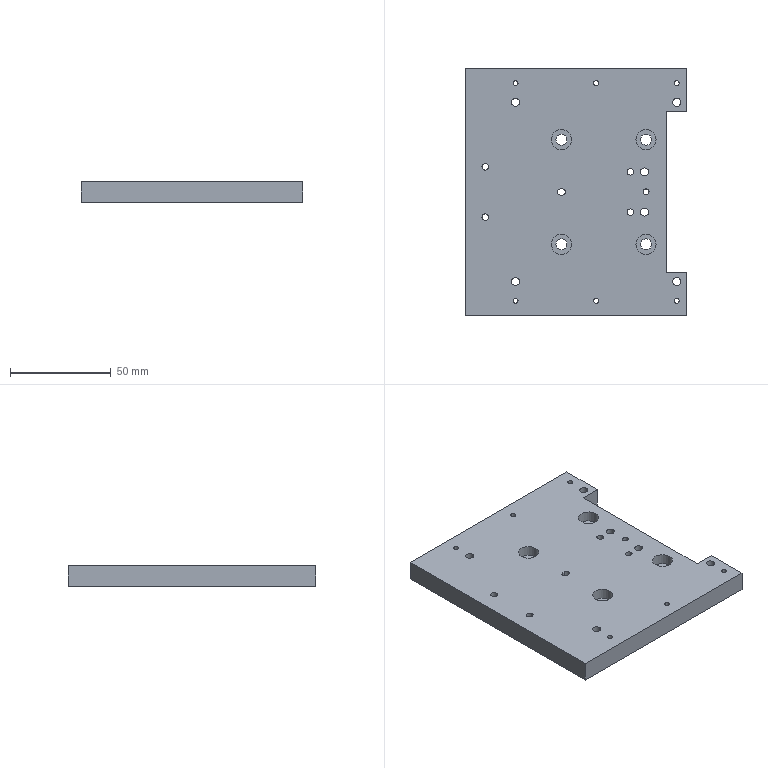Part | 1 solid | 43 faces | box 110 x 123 x 10 mm | volume 123604 mm3 | cylinder 27 | plane 16 | commonest cylinder face diameters 2.5 x6 4 x6 3.3 x4 5.5 x4 10 x4 3 x3
STEP:
#1=CARTESIAN_POINT('',(48.25,60.,10.));
#2=VERTEX_POINT('',#1);
#3=CARTESIAN_POINT('',(48.25,60.,0.));
#4=VERTEX_POINT('',#3);
#5=CARTESIAN_POINT('',(48.25,60.,10.));
#6=DIRECTION('',(0.,0.,-1.));
#7=VECTOR('',#6,1000.);
#8=LINE('',#5,#7);
#9=EDGE_CURVE('',#2,#4,#8,.T.);
#10=ORIENTED_EDGE('',*,*,#9,.T.);
#11=CARTESIAN_POINT('',(47.25,60.,0.));
#12=VERTEX_POINT('',#11);
#13=CARTESIAN_POINT('',(47.25,60.,0.));
#14=DIRECTION('',(1.,0.,0.));
#15=VECTOR('',#14,1000.);
#16=LINE('',#13,#15);
#17=EDGE_CURVE('',#12,#4,#16,.T.);
#18=ORIENTED_EDGE('',*,*,#17,.F.);
#19=CARTESIAN_POINT('',(47.25,60.,10.));
#20=VERTEX_POINT('',#19);
#21=CARTESIAN_POINT('',(47.25,60.,10.));
#22=DIRECTION('',(0.,0.,1.));
#23=VECTOR('',#22,1000.);
#24=LINE('',#21,#23);
#25=EDGE_CURVE('',#12,#20,#24,.T.);
#26=ORIENTED_EDGE('',*,*,#25,.T.);
#27=CARTESIAN_POINT('',(47.25,60.,10.));
#28=DIRECTION('',(1.,0.,0.));
#29=VECTOR('',#28,1000.);
#30=LINE('',#27,#29);
#31=EDGE_CURVE('',#20,#2,#30,.T.);
#32=ORIENTED_EDGE('',*,*,#31,.T.);
#33=EDGE_LOOP('',(#10,#18,#26,#32));
#34=FACE_BOUND('',#33,.T.);
#35=CARTESIAN_POINT('',(47.25,60.,10.));
#36=DIRECTION('',(0.,-1.,0.));
#37=DIRECTION('',(0.,0.,-1.));
#38=AXIS2_PLACEMENT_3D('',#35,#36,#37);
#39=PLANE('',#38);
#40=ADVANCED_FACE('',(#34),#39,.F.);
#41=CARTESIAN_POINT('',(48.25,63.,0.));
#42=VERTEX_POINT('',#41);
#43=CARTESIAN_POINT('',(48.25,63.,10.));
#44=VERTEX_POINT('',#43);
#45=CARTESIAN_POINT('',(48.25,63.,10.));
#46=DIRECTION('',(0.,0.,1.));
#47=VECTOR('',#46,1000.);
#48=LINE('',#45,#47);
#49=EDGE_CURVE('',#42,#44,#48,.T.);
#50=ORIENTED_EDGE('',*,*,#49,.T.);
#51=CARTESIAN_POINT('',(47.25,63.,10.));
#52=VERTEX_POINT('',#51);
#53=CARTESIAN_POINT('',(47.25,63.,10.));
#54=DIRECTION('',(1.,0.,0.));
#55=VECTOR('',#54,1000.);
#56=LINE('',#53,#55);
#57=EDGE_CURVE('',#52,#44,#56,.T.);
#58=ORIENTED_EDGE('',*,*,#57,.F.);
#59=CARTESIAN_POINT('',(47.25,63.,0.));
#60=VERTEX_POINT('',#59);
#61=CARTESIAN_POINT('',(47.25,63.,10.));
#62=DIRECTION('',(0.,0.,-1.));
#63=VECTOR('',#62,1000.);
#64=LINE('',#61,#63);
#65=EDGE_CURVE('',#52,#60,#64,.T.);
#66=ORIENTED_EDGE('',*,*,#65,.T.);
#67=CARTESIAN_POINT('',(47.25,63.,0.));
#68=DIRECTION('',(1.,0.,0.));
#69=VECTOR('',#68,1000.);
#70=LINE('',#67,#69);
#71=EDGE_CURVE('',#60,#42,#70,.T.);
#72=ORIENTED_EDGE('',*,*,#71,.T.);
#73=EDGE_LOOP('',(#50,#58,#66,#72));
#74=FACE_BOUND('',#73,.T.);
#75=CARTESIAN_POINT('',(47.25,63.,10.));
#76=DIRECTION('',(0.,1.,0.));
#77=DIRECTION('',(0.,0.,1.));
#78=AXIS2_PLACEMENT_3D('',#75,#76,#77);
#79=PLANE('',#78);
#80=ADVANCED_FACE('',(#74),#79,.F.);
#81=CARTESIAN_POINT('',(47.25,61.5,10.));
#82=DIRECTION('',(0.,0.,1.));
#83=DIRECTION('',(1.,0.,0.));
#84=AXIS2_PLACEMENT_3D('',#81,#82,#83);
#85=CIRCLE('',#84,1.5);
#86=EDGE_CURVE('',#52,#20,#85,.T.);
#87=ORIENTED_EDGE('',*,*,#86,.T.);
#88=ORIENTED_EDGE('',*,*,#25,.F.);
#89=CARTESIAN_POINT('',(47.25,61.5,0.));
#90=DIRECTION('',(0.,0.,1.));
#91=DIRECTION('',(1.,0.,0.));
#92=AXIS2_PLACEMENT_3D('',#89,#90,#91);
#93=CIRCLE('',#92,1.5);
#94=EDGE_CURVE('',#60,#12,#93,.T.);
#95=ORIENTED_EDGE('',*,*,#94,.F.);
#96=ORIENTED_EDGE('',*,*,#65,.F.);
#97=EDGE_LOOP('',(#87,#88,#95,#96));
#98=FACE_BOUND('',#97,.T.);
#99=CARTESIAN_POINT('',(47.25,61.5,10.));
#100=DIRECTION('',(0.,0.,1.));
#101=DIRECTION('',(1.,0.,0.));
#102=AXIS2_PLACEMENT_3D('',#99,#100,#101);
#103=CYLINDRICAL_SURFACE('',#102,1.5);
#104=ADVANCED_FACE('',(#98),#103,.F.);
#105=CARTESIAN_POINT('',(110.,101.5,10.));
#106=VERTEX_POINT('',#105);
#107=CARTESIAN_POINT('',(100.,101.5,10.));
#108=VERTEX_POINT('',#107);
#109=CARTESIAN_POINT('',(110.,101.5,10.));
#110=DIRECTION('',(-1.,0.,0.));
#111=VECTOR('',#110,1000.);
#112=LINE('',#109,#111);
#113=EDGE_CURVE('',#106,#108,#112,.T.);
#114=ORIENTED_EDGE('',*,*,#113,.T.);
#115=CARTESIAN_POINT('',(100.,101.5,0.));
#116=VERTEX_POINT('',#115);
#117=CARTESIAN_POINT('',(100.,101.5,0.));
#118=DIRECTION('',(0.,0.,1.));
#119=VECTOR('',#118,1000.);
#120=LINE('',#117,#119);
#121=EDGE_CURVE('',#116,#108,#120,.T.);
#122=ORIENTED_EDGE('',*,*,#121,.F.);
#123=CARTESIAN_POINT('',(110.,101.5,0.));
#124=VERTEX_POINT('',#123);
#125=CARTESIAN_POINT('',(110.,101.5,0.));
#126=DIRECTION('',(-1.,0.,0.));
#127=VECTOR('',#126,1000.);
#128=LINE('',#125,#127);
#129=EDGE_CURVE('',#124,#116,#128,.T.);
#130=ORIENTED_EDGE('',*,*,#129,.F.);
#131=CARTESIAN_POINT('',(110.,101.5,0.));
#132=DIRECTION('',(0.,0.,1.));
#133=VECTOR('',#132,1000.);
#134=LINE('',#131,#133);
#135=EDGE_CURVE('',#124,#106,#134,.T.);
#136=ORIENTED_EDGE('',*,*,#135,.T.);
#137=EDGE_LOOP('',(#114,#122,#130,#136));
#138=FACE_BOUND('',#137,.T.);
#139=CARTESIAN_POINT('',(110.,101.5,0.));
#140=DIRECTION('',(0.,1.,0.));
#141=DIRECTION('',(0.,0.,1.));
#142=AXIS2_PLACEMENT_3D('',#139,#140,#141);
#143=PLANE('',#142);
#144=ADVANCED_FACE('',(#138),#143,.F.);
#145=CARTESIAN_POINT('',(100.,21.5,10.));
#146=VERTEX_POINT('',#145);
#147=CARTESIAN_POINT('',(100.,101.5,10.));
#148=DIRECTION('',(0.,-1.,0.));
#149=VECTOR('',#148,1000.);
#150=LINE('',#147,#149);
#151=EDGE_CURVE('',#108,#146,#150,.T.);
#152=ORIENTED_EDGE('',*,*,#151,.T.);
#153=CARTESIAN_POINT('',(100.,21.5,0.));
#154=VERTEX_POINT('',#153);
#155=CARTESIAN_POINT('',(100.,21.5,0.));
#156=DIRECTION('',(0.,0.,1.));
#157=VECTOR('',#156,1000.);
#158=LINE('',#155,#157);
#159=EDGE_CURVE('',#154,#146,#158,.T.);
#160=ORIENTED_EDGE('',*,*,#159,.F.);
#161=CARTESIAN_POINT('',(100.,101.5,0.));
#162=DIRECTION('',(0.,-1.,0.));
#163=VECTOR('',#162,1000.);
#164=LINE('',#161,#163);
#165=EDGE_CURVE('',#116,#154,#164,.T.);
#166=ORIENTED_EDGE('',*,*,#165,.F.);
#167=ORIENTED_EDGE('',*,*,#121,.T.);
#168=EDGE_LOOP('',(#152,#160,#166,#167));
#169=FACE_BOUND('',#168,.T.);
#170=CARTESIAN_POINT('',(100.,101.5,0.));
#171=DIRECTION('',(-1.,0.,0.));
#172=DIRECTION('',(0.,0.,1.));
#173=AXIS2_PLACEMENT_3D('',#170,#171,#172);
#174=PLANE('',#173);
#175=ADVANCED_FACE('',(#169),#174,.F.);
#176=CARTESIAN_POINT('',(110.,21.5,10.));
#177=VERTEX_POINT('',#176);
#178=CARTESIAN_POINT('',(110.,21.5,10.));
#179=DIRECTION('',(1.,0.,0.));
#180=VECTOR('',#179,1000.);
#181=LINE('',#178,#180);
#182=EDGE_CURVE('',#146,#177,#181,.T.);
#183=ORIENTED_EDGE('',*,*,#182,.T.);
#184=CARTESIAN_POINT('',(110.,21.5,0.));
#185=VERTEX_POINT('',#184);
#186=CARTESIAN_POINT('',(110.,21.5,0.));
#187=DIRECTION('',(0.,0.,1.));
#188=VECTOR('',#187,1000.);
#189=LINE('',#186,#188);
#190=EDGE_CURVE('',#185,#177,#189,.T.);
#191=ORIENTED_EDGE('',*,*,#190,.F.);
#192=CARTESIAN_POINT('',(110.,21.5,0.));
#193=DIRECTION('',(1.,0.,0.));
#194=VECTOR('',#193,1000.);
#195=LINE('',#192,#194);
#196=EDGE_CURVE('',#154,#185,#195,.T.);
#197=ORIENTED_EDGE('',*,*,#196,.F.);
#198=ORIENTED_EDGE('',*,*,#159,.T.);
#199=EDGE_LOOP('',(#183,#191,#197,#198));
#200=FACE_BOUND('',#199,.T.);
#201=CARTESIAN_POINT('',(110.,21.5,0.));
#202=DIRECTION('',(0.,-1.,0.));
#203=DIRECTION('',(0.,0.,-1.));
#204=AXIS2_PLACEMENT_3D('',#201,#202,#203);
#205=PLANE('',#204);
#206=ADVANCED_FACE('',(#200),#205,.F.);
#207=CARTESIAN_POINT('',(52.75,87.5,4.6));
#208=VERTEX_POINT('',#207);
#209=CARTESIAN_POINT('',(47.75,87.5,4.6));
#210=DIRECTION('',(0.,0.,1.));
#211=DIRECTION('',(1.,0.,0.));
#212=AXIS2_PLACEMENT_3D('',#209,#210,#211);
#213=CIRCLE('',#212,5.);
#214=EDGE_CURVE('',#208,#208,#213,.T.);
#215=ORIENTED_EDGE('',*,*,#214,.T.);
#216=EDGE_LOOP('',(#215));
#217=FACE_BOUND('',#216,.T.);
#218=CARTESIAN_POINT('',(50.5,87.5,4.6));
#219=VERTEX_POINT('',#218);
#220=CARTESIAN_POINT('',(47.75,87.5,4.6));
#221=DIRECTION('',(0.,0.,1.));
#222=DIRECTION('',(1.,0.,0.));
#223=AXIS2_PLACEMENT_3D('',#220,#221,#222);
#224=CIRCLE('',#223,2.75);
#225=EDGE_CURVE('',#219,#219,#224,.T.);
#226=ORIENTED_EDGE('',*,*,#225,.F.);
#227=EDGE_LOOP('',(#226));
#228=FACE_BOUND('',#227,.T.);
#229=CARTESIAN_POINT('',(50.5,87.5,4.6));
#230=DIRECTION('',(0.,0.,-1.));
#231=DIRECTION('',(-1.,0.,0.));
#232=AXIS2_PLACEMENT_3D('',#229,#230,#231);
#233=PLANE('',#232);
#234=ADVANCED_FACE('',(#217,#228),#233,.F.);
#235=CARTESIAN_POINT('',(42.75,35.5,4.6));
#236=VERTEX_POINT('',#235);
#237=CARTESIAN_POINT('',(47.75,35.5,4.6));
#238=DIRECTION('',(0.,0.,1.));
#239=DIRECTION('',(-1.,0.,0.));
#240=AXIS2_PLACEMENT_3D('',#237,#238,#239);
#241=CIRCLE('',#240,5.);
#242=EDGE_CURVE('',#236,#236,#241,.T.);
#243=ORIENTED_EDGE('',*,*,#242,.T.);
#244=EDGE_LOOP('',(#243));
#245=FACE_BOUND('',#244,.T.);
#246=CARTESIAN_POINT('',(45.,35.5,4.6));
#247=VERTEX_POINT('',#246);
#248=CARTESIAN_POINT('',(47.75,35.5,4.6));
#249=DIRECTION('',(0.,0.,1.));
#250=DIRECTION('',(-1.,0.,0.));
#251=AXIS2_PLACEMENT_3D('',#248,#249,#250);
#252=CIRCLE('',#251,2.75);
#253=EDGE_CURVE('',#247,#247,#252,.T.);
#254=ORIENTED_EDGE('',*,*,#253,.F.);
#255=EDGE_LOOP('',(#254));
#256=FACE_BOUND('',#255,.T.);
#257=CARTESIAN_POINT('',(50.5,87.5,4.6));
#258=DIRECTION('',(0.,0.,-1.));
#259=DIRECTION('',(-1.,0.,0.));
#260=AXIS2_PLACEMENT_3D('',#257,#258,#259);
#261=PLANE('',#260);
#262=ADVANCED_FACE('',(#245,#256),#261,.F.);
#263=CARTESIAN_POINT('',(84.75,87.5,4.6));
#264=VERTEX_POINT('',#263);
#265=CARTESIAN_POINT('',(89.75,87.5,4.6));
#266=DIRECTION('',(0.,0.,1.));
#267=DIRECTION('',(-1.,0.,0.));
#268=AXIS2_PLACEMENT_3D('',#265,#266,#267);
#269=CIRCLE('',#268,5.);
#270=EDGE_CURVE('',#264,#264,#269,.T.);
#271=ORIENTED_EDGE('',*,*,#270,.T.);
#272=EDGE_LOOP('',(#271));
#273=FACE_BOUND('',#272,.T.);
#274=CARTESIAN_POINT('',(87.,87.5,4.6));
#275=VERTEX_POINT('',#274);
#276=CARTESIAN_POINT('',(89.75,87.5,4.6));
#277=DIRECTION('',(0.,0.,1.));
#278=DIRECTION('',(-1.,0.,0.));
#279=AXIS2_PLACEMENT_3D('',#276,#277,#278);
#280=CIRCLE('',#279,2.75);
#281=EDGE_CURVE('',#275,#275,#280,.T.);
#282=ORIENTED_EDGE('',*,*,#281,.F.);
#283=EDGE_LOOP('',(#282));
#284=FACE_BOUND('',#283,.T.);
#285=CARTESIAN_POINT('',(50.5,87.5,4.6));
#286=DIRECTION('',(0.,0.,-1.));
#287=DIRECTION('',(-1.,0.,0.));
#288=AXIS2_PLACEMENT_3D('',#285,#286,#287);
#289=PLANE('',#288);
#290=ADVANCED_FACE('',(#273,#284),#289,.F.);
#291=CARTESIAN_POINT('',(84.75,35.5,4.6));
#292=VERTEX_POINT('',#291);
#293=CARTESIAN_POINT('',(89.75,35.5,4.6));
#294=DIRECTION('',(0.,0.,1.));
#295=DIRECTION('',(-1.,0.,0.));
#296=AXIS2_PLACEMENT_3D('',#293,#294,#295);
#297=CIRCLE('',#296,5.);
#298=EDGE_CURVE('',#292,#292,#297,.T.);
#299=ORIENTED_EDGE('',*,*,#298,.T.);
#300=EDGE_LOOP('',(#299));
#301=FACE_BOUND('',#300,.T.);
#302=CARTESIAN_POINT('',(87.,35.5,4.6));
#303=VERTEX_POINT('',#302);
#304=CARTESIAN_POINT('',(89.75,35.5,4.6));
#305=DIRECTION('',(0.,0.,1.));
#306=DIRECTION('',(-1.,0.,0.));
#307=AXIS2_PLACEMENT_3D('',#304,#305,#306);
#308=CIRCLE('',#307,2.75);
#309=EDGE_CURVE('',#303,#303,#308,.T.);
#310=ORIENTED_EDGE('',*,*,#309,.F.);
#311=EDGE_LOOP('',(#310));
#312=FACE_BOUND('',#311,.T.);
#313=CARTESIAN_POINT('',(50.5,87.5,4.6));
#314=DIRECTION('',(0.,0.,-1.));
#315=DIRECTION('',(-1.,0.,0.));
#316=AXIS2_PLACEMENT_3D('',#313,#314,#315);
#317=PLANE('',#316);
#318=ADVANCED_FACE('',(#301,#312),#317,.F.);
#319=CARTESIAN_POINT('',(110.,123.,0.));
#320=VERTEX_POINT('',#319);
#321=CARTESIAN_POINT('',(0.,123.,0.));
#322=VERTEX_POINT('',#321);
#323=CARTESIAN_POINT('',(0.,123.,0.));
#324=DIRECTION('',(-1.,0.,0.));
#325=VECTOR('',#324,1000.);
#326=LINE('',#323,#325);
#327=EDGE_CURVE('',#320,#322,#326,.T.);
#328=ORIENTED_EDGE('',*,*,#327,.T.);
#329=CARTESIAN_POINT('',(0.,123.,10.));
#330=VERTEX_POINT('',#329);
#331=CARTESIAN_POINT('',(0.,123.,10.));
#332=DIRECTION('',(0.,0.,-1.));
#333=VECTOR('',#332,1000.);
#334=LINE('',#331,#333);
#335=EDGE_CURVE('',#330,#322,#334,.T.);
#336=ORIENTED_EDGE('',*,*,#335,.F.);
#337=CARTESIAN_POINT('',(110.,123.,10.));
#338=VERTEX_POINT('',#337);
#339=CARTESIAN_POINT('',(0.,123.,10.));
#340=DIRECTION('',(-1.,0.,0.));
#341=VECTOR('',#340,1000.);
#342=LINE('',#339,#341);
#343=EDGE_CURVE('',#338,#330,#342,.T.);
#344=ORIENTED_EDGE('',*,*,#343,.F.);
#345=CARTESIAN_POINT('',(110.,123.,10.));
#346=DIRECTION('',(0.,0.,-1.));
#347=VECTOR('',#346,1000.);
#348=LINE('',#345,#347);
#349=EDGE_CURVE('',#338,#320,#348,.T.);
#350=ORIENTED_EDGE('',*,*,#349,.T.);
#351=EDGE_LOOP('',(#328,#336,#344,#350));
#352=FACE_BOUND('',#351,.T.);
#353=CARTESIAN_POINT('',(0.,123.,10.));
#354=DIRECTION('',(0.,-1.,0.));
#355=DIRECTION('',(0.,0.,-1.));
#356=AXIS2_PLACEMENT_3D('',#353,#354,#355);
#357=PLANE('',#356);
#358=ADVANCED_FACE('',(#352),#357,.F.);
#359=CARTESIAN_POINT('',(110.,0.,10.));
#360=DIRECTION('',(0.,1.,0.));
#361=VECTOR('',#360,1000.);
#362=LINE('',#359,#361);
#363=EDGE_CURVE('',#106,#338,#362,.T.);
#364=ORIENTED_EDGE('',*,*,#363,.F.);
#365=ORIENTED_EDGE('',*,*,#135,.F.);
#366=CARTESIAN_POINT('',(110.,0.,0.));
#367=DIRECTION('',(0.,1.,0.));
#368=VECTOR('',#367,1000.);
#369=LINE('',#366,#368);
#370=EDGE_CURVE('',#124,#320,#369,.T.);
#371=ORIENTED_EDGE('',*,*,#370,.T.);
#372=ORIENTED_EDGE('',*,*,#349,.F.);
#373=EDGE_LOOP('',(#364,#365,#371,#372));
#374=FACE_BOUND('',#373,.T.);
#375=CARTESIAN_POINT('',(110.,0.,10.));
#376=DIRECTION('',(-1.,0.,0.));
#377=DIRECTION('',(0.,0.,1.));
#378=AXIS2_PLACEMENT_3D('',#375,#376,#377);
#379=PLANE('',#378);
#380=ADVANCED_FACE('',(#374),#379,.F.);
#381=CARTESIAN_POINT('',(0.,0.,0.));
#382=VERTEX_POINT('',#381);
#383=CARTESIAN_POINT('',(110.,0.,0.));
#384=VERTEX_POINT('',#383);
#385=CARTESIAN_POINT('',(0.,0.,0.));
#386=DIRECTION('',(1.,0.,0.));
#387=VECTOR('',#386,1000.);
#388=LINE('',#385,#387);
#389=EDGE_CURVE('',#382,#384,#388,.T.);
#390=ORIENTED_EDGE('',*,*,#389,.T.);
#391=CARTESIAN_POINT('',(110.,0.,10.));
#392=VERTEX_POINT('',#391);
#393=CARTESIAN_POINT('',(110.,0.,10.));
#394=DIRECTION('',(0.,0.,-1.));
#395=VECTOR('',#394,1000.);
#396=LINE('',#393,#395);
#397=EDGE_CURVE('',#392,#384,#396,.T.);
#398=ORIENTED_EDGE('',*,*,#397,.F.);
#399=CARTESIAN_POINT('',(0.,0.,10.));
#400=VERTEX_POINT('',#399);
#401=CARTESIAN_POINT('',(0.,0.,10.));
#402=DIRECTION('',(1.,0.,0.));
#403=VECTOR('',#402,1000.);
#404=LINE('',#401,#403);
#405=EDGE_CURVE('',#400,#392,#404,.T.);
#406=ORIENTED_EDGE('',*,*,#405,.F.);
#407=CARTESIAN_POINT('',(0.,0.,10.));
#408=DIRECTION('',(0.,0.,-1.));
#409=VECTOR('',#408,1000.);
#410=LINE('',#407,#409);
#411=EDGE_CURVE('',#400,#382,#410,.T.);
#412=ORIENTED_EDGE('',*,*,#411,.T.);
#413=EDGE_LOOP('',(#390,#398,#406,#412));
#414=FACE_BOUND('',#413,.T.);
#415=CARTESIAN_POINT('',(0.,0.,10.));
#416=DIRECTION('',(0.,1.,0.));
#417=DIRECTION('',(0.,0.,1.));
#418=AXIS2_PLACEMENT_3D('',#415,#416,#417);
#419=PLANE('',#418);
#420=ADVANCED_FACE('',(#414),#419,.F.);
#421=CARTESIAN_POINT('',(0.,0.,0.));
#422=DIRECTION('',(0.,-1.,0.));
#423=VECTOR('',#422,1000.);
#424=LINE('',#421,#423);
#425=EDGE_CURVE('',#322,#382,#424,.T.);
#426=ORIENTED_EDGE('',*,*,#425,.T.);
#427=ORIENTED_EDGE('',*,*,#411,.F.);
#428=CARTESIAN_POINT('',(0.,0.,10.));
#429=DIRECTION('',(0.,-1.,0.));
#430=VECTOR('',#429,1000.);
#431=LINE('',#428,#430);
#432=EDGE_CURVE('',#330,#400,#431,.T.);
#433=ORIENTED_EDGE('',*,*,#432,.F.);
#434=ORIENTED_EDGE('',*,*,#335,.T.);
#435=EDGE_LOOP('',(#426,#427,#433,#434));
#436=FACE_BOUND('',#435,.T.);
#437=CARTESIAN_POINT('',(0.,0.,10.));
#438=DIRECTION('',(1.,0.,0.));
#439=DIRECTION('',(0.,0.,-1.));
#440=AXIS2_PLACEMENT_3D('',#437,#438,#439);
#441=PLANE('',#440);
#442=ADVANCED_FACE('',(#436),#441,.F.);
#443=CARTESIAN_POINT('',(94.75,87.5,10.));
#444=VERTEX_POINT('',#443);
#445=CARTESIAN_POINT('',(89.75,87.5,10.));
#446=DIRECTION('',(0.,0.,1.));
#447=DIRECTION('',(1.,0.,0.));
#448=AXIS2_PLACEMENT_3D('',#445,#446,#447);
#449=CIRCLE('',#448,5.);
#450=EDGE_CURVE('',#444,#444,#449,.T.);
#451=ORIENTED_EDGE('',*,*,#450,.F.);
#452=EDGE_LOOP('',(#451));
#453=FACE_BOUND('',#452,.T.);
#454=CARTESIAN_POINT('',(110.,0.,10.));
#455=DIRECTION('',(0.,1.,0.));
#456=VECTOR('',#455,1000.);
#457=LINE('',#454,#456);
#458=EDGE_CURVE('',#392,#177,#457,.T.);
#459=ORIENTED_EDGE('',*,*,#458,.T.);
#460=ORIENTED_EDGE('',*,*,#182,.F.);
#461=ORIENTED_EDGE('',*,*,#151,.F.);
#462=ORIENTED_EDGE('',*,*,#113,.F.);
#463=ORIENTED_EDGE('',*,*,#363,.T.);
#464=ORIENTED_EDGE('',*,*,#343,.T.);
#465=ORIENTED_EDGE('',*,*,#432,.T.);
#466=ORIENTED_EDGE('',*,*,#405,.T.);
#467=EDGE_LOOP('',(#459,#460,#461,#462,#463,#464,#465,#466));
#468=FACE_BOUND('',#467,.T.);
#469=CARTESIAN_POINT('',(106.25,7.5,10.));
#470=VERTEX_POINT('',#469);
#471=CARTESIAN_POINT('',(105.,7.5,10.));
#472=DIRECTION('',(0.,0.,1.));
#473=DIRECTION('',(1.,0.,0.));
#474=AXIS2_PLACEMENT_3D('',#471,#472,#473);
#475=CIRCLE('',#474,1.25);
#476=EDGE_CURVE('',#470,#470,#475,.T.);
#477=ORIENTED_EDGE('',*,*,#476,.F.);
#478=EDGE_LOOP('',(#477));
#479=FACE_BOUND('',#478,.T.);
#480=CARTESIAN_POINT('',(66.25,7.5,10.));
#481=VERTEX_POINT('',#480);
#482=CARTESIAN_POINT('',(65.,7.5,10.));
#483=DIRECTION('',(0.,0.,1.));
#484=DIRECTION('',(1.,0.,0.));
#485=AXIS2_PLACEMENT_3D('',#482,#483,#484);
#486=CIRCLE('',#485,1.25);
#487=EDGE_CURVE('',#481,#481,#486,.T.);
#488=ORIENTED_EDGE('',*,*,#487,.F.);
#489=EDGE_LOOP('',(#488));
#490=FACE_BOUND('',#489,.T.);
#491=CARTESIAN_POINT('',(26.25,7.5,10.));
#492=VERTEX_POINT('',#491);
#493=CARTESIAN_POINT('',(25.,7.5,10.));
#494=DIRECTION('',(0.,0.,1.));
#495=DIRECTION('',(1.,0.,0.));
#496=AXIS2_PLACEMENT_3D('',#493,#494,#495);
#497=CIRCLE('',#496,1.25);
#498=EDGE_CURVE('',#492,#492,#497,.T.);
#499=ORIENTED_EDGE('',*,*,#498,.F.);
#500=EDGE_LOOP('',(#499));
#501=FACE_BOUND('',#500,.T.);
#502=CARTESIAN_POINT('',(26.25,115.5,10.));
#503=VERTEX_POINT('',#502);
#504=CARTESIAN_POINT('',(25.,115.5,10.));
#505=DIRECTION('',(0.,0.,1.));
#506=DIRECTION('',(1.,0.,0.));
#507=AXIS2_PLACEMENT_3D('',#504,#505,#506);
#508=CIRCLE('',#507,1.25);
#509=EDGE_CURVE('',#503,#503,#508,.T.);
#510=ORIENTED_EDGE('',*,*,#509,.F.);
#511=EDGE_LOOP('',(#510));
#512=FACE_BOUND('',#511,.T.);
#513=CARTESIAN_POINT('',(66.25,115.5,10.));
#514=VERTEX_POINT('',#513);
#515=CARTESIAN_POINT('',(65.,115.5,10.));
#516=DIRECTION('',(0.,0.,1.));
#517=DIRECTION('',(1.,0.,0.));
#518=AXIS2_PLACEMENT_3D('',#515,#516,#517);
#519=CIRCLE('',#518,1.25);
#520=EDGE_CURVE('',#514,#514,#519,.T.);
#521=ORIENTED_EDGE('',*,*,#520,.F.);
#522=EDGE_LOOP('',(#521));
#523=FACE_BOUND('',#522,.T.);
#524=CARTESIAN_POINT('',(106.25,115.5,10.));
#525=VERTEX_POINT('',#524);
#526=CARTESIAN_POINT('',(105.,115.5,10.));
#527=DIRECTION('',(0.,0.,1.));
#528=DIRECTION('',(1.,0.,0.));
#529=AXIS2_PLACEMENT_3D('',#526,#527,#528);
#530=CIRCLE('',#529,1.25);
#531=EDGE_CURVE('',#525,#525,#530,.T.);
#532=ORIENTED_EDGE('',*,*,#531,.F.);
#533=EDGE_LOOP('',(#532));
#534=FACE_BOUND('',#533,.T.);
#535=CARTESIAN_POINT('',(94.75,35.5,10.));
#536=VERTEX_POINT('',#535);
#537=CARTESIAN_POINT('',(89.75,35.5,10.));
#538=DIRECTION('',(0.,0.,1.));
#539=DIRECTION('',(1.,0.,0.));
#540=AXIS2_PLACEMENT_3D('',#537,#538,#539);
#541=CIRCLE('',#540,5.);
#542=EDGE_CURVE('',#536,#536,#541,.T.);
#543=ORIENTED_EDGE('',*,*,#542,.F.);
#544=EDGE_LOOP('',(#543));
#545=FACE_BOUND('',#544,.T.);
#546=CARTESIAN_POINT('',(52.75,35.5,10.));
#547=VERTEX_POINT('',#546);
#548=CARTESIAN_POINT('',(47.75,35.5,10.));
#549=DIRECTION('',(0.,0.,1.));
#550=DIRECTION('',(1.,0.,0.));
#551=AXIS2_PLACEMENT_3D('',#548,#549,#550);
#552=CIRCLE('',#551,5.);
#553=EDGE_CURVE('',#547,#547,#552,.T.);
#554=ORIENTED_EDGE('',*,*,#553,.F.);
#555=EDGE_LOOP('',(#554));
#556=FACE_BOUND('',#555,.T.);
#557=CARTESIAN_POINT('',(52.75,87.5,10.));
#558=VERTEX_POINT('',#557);
#559=CARTESIAN_POINT('',(47.75,87.5,10.));
#560=DIRECTION('',(0.,0.,1.));
#561=DIRECTION('',(1.,0.,0.));
#562=AXIS2_PLACEMENT_3D('',#559,#560,#561);
#563=CIRCLE('',#562,5.);
#564=EDGE_CURVE('',#558,#558,#563,.T.);
#565=ORIENTED_EDGE('',*,*,#564,.F.);
#566=EDGE_LOOP('',(#565));
#567=FACE_BOUND('',#566,.T.);
#568=CARTESIAN_POINT('',(11.65,49.,10.));
#569=VERTEX_POINT('',#568);
#570=CARTESIAN_POINT('',(10.,49.,10.));
#571=DIRECTION('',(0.,0.,1.));
#572=DIRECTION('',(1.,0.,0.));
#573=AXIS2_PLACEMENT_3D('',#570,#571,#572);
#574=CIRCLE('',#573,1.65);
#575=EDGE_CURVE('',#569,#569,#574,.T.);
#576=ORIENTED_EDGE('',*,*,#575,.F.);
#577=EDGE_LOOP('',(#576));
#578=FACE_BOUND('',#577,.T.);
#579=CARTESIAN_POINT('',(11.65,74.,10.));
#580=VERTEX_POINT('',#579);
#581=CARTESIAN_POINT('',(10.,74.,10.));
#582=DIRECTION('',(0.,0.,1.));
#583=DIRECTION('',(1.,0.,0.));
#584=AXIS2_PLACEMENT_3D('',#581,#582,#583);
#585=CIRCLE('',#584,1.65);
#586=EDGE_CURVE('',#580,#580,#585,.T.);
#587=ORIENTED_EDGE('',*,*,#586,.F.);
#588=EDGE_LOOP('',(#587));
#589=FACE_BOUND('',#588,.T.);
#590=CARTESIAN_POINT('',(83.65,51.5,10.));
#591=VERTEX_POINT('',#590);
#592=CARTESIAN_POINT('',(82.,51.5,10.));
#593=DIRECTION('',(0.,0.,1.));
#594=DIRECTION('',(1.,0.,0.));
#595=AXIS2_PLACEMENT_3D('',#592,#593,#594);
#596=CIRCLE('',#595,1.65);
#597=EDGE_CURVE('',#591,#591,#596,.T.);
#598=ORIENTED_EDGE('',*,*,#597,.F.);
#599=EDGE_LOOP('',(#598));
#600=FACE_BOUND('',#599,.T.);
#601=CARTESIAN_POINT('',(83.65,71.5,10.));
#602=VERTEX_POINT('',#601);
#603=CARTESIAN_POINT('',(82.,71.5,10.));
#604=DIRECTION('',(0.,0.,1.));
#605=DIRECTION('',(1.,0.,0.));
#606=AXIS2_PLACEMENT_3D('',#603,#604,#605);
#607=CIRCLE('',#606,1.65);
#608=EDGE_CURVE('',#602,#602,#607,.T.);
#609=ORIENTED_EDGE('',*,*,#608,.F.);
#610=EDGE_LOOP('',(#609));
#611=FACE_BOUND('',#610,.T.);
#612=CARTESIAN_POINT('',(91.,51.5,10.));
#613=VERTEX_POINT('',#612);
#614=CARTESIAN_POINT('',(89.,51.5,10.));
#615=DIRECTION('',(0.,0.,1.));
#616=DIRECTION('',(1.,0.,0.));
#617=AXIS2_PLACEMENT_3D('',#614,#615,#616);
#618=CIRCLE('',#617,2.);
#619=EDGE_CURVE('',#613,#613,#618,.T.);
#620=ORIENTED_EDGE('',*,*,#619,.F.);
#621=EDGE_LOOP('',(#620));
#622=FACE_BOUND('',#621,.T.);
#623=CARTESIAN_POINT('',(91.,71.5,10.));
#624=VERTEX_POINT('',#623);
#625=CARTESIAN_POINT('',(89.,71.5,10.));
#626=DIRECTION('',(0.,0.,1.));
#627=DIRECTION('',(1.,0.,0.));
#628=AXIS2_PLACEMENT_3D('',#625,#626,#627);
#629=CIRCLE('',#628,2.);
#630=EDGE_CURVE('',#624,#624,#629,.T.);
#631=ORIENTED_EDGE('',*,*,#630,.F.);
#632=EDGE_LOOP('',(#631));
#633=FACE_BOUND('',#632,.T.);
#634=CARTESIAN_POINT('',(27.,17.,10.));
#635=VERTEX_POINT('',#634);
#636=CARTESIAN_POINT('',(25.,17.,10.));
#637=DIRECTION('',(0.,0.,1.));
#638=DIRECTION('',(1.,0.,0.));
#639=AXIS2_PLACEMENT_3D('',#636,#637,#638);
#640=CIRCLE('',#639,2.);
#641=EDGE_CURVE('',#635,#635,#640,.T.);
#642=ORIENTED_EDGE('',*,*,#641,.F.);
#643=EDGE_LOOP('',(#642));
#644=FACE_BOUND('',#643,.T.);
#645=CARTESIAN_POINT('',(107.,17.,10.));
#646=VERTEX_POINT('',#645);
#647=CARTESIAN_POINT('',(105.,17.,10.));
#648=DIRECTION('',(0.,0.,1.));
#649=DIRECTION('',(1.,0.,0.));
#650=AXIS2_PLACEMENT_3D('',#647,#648,#649);
#651=CIRCLE('',#650,2.);
#652=EDGE_CURVE('',#646,#646,#651,.T.);
#653=ORIENTED_EDGE('',*,*,#652,.F.);
#654=EDGE_LOOP('',(#653));
#655=FACE_BOUND('',#654,.T.);
#656=CARTESIAN_POINT('',(27.,106.,10.));
#657=VERTEX_POINT('',#656);
#658=CARTESIAN_POINT('',(25.,106.,10.));
#659=DIRECTION('',(0.,0.,1.));
#660=DIRECTION('',(1.,0.,0.));
#661=AXIS2_PLACEMENT_3D('',#658,#659,#660);
#662=CIRCLE('',#661,2.);
#663=EDGE_CURVE('',#657,#657,#662,.T.);
#664=ORIENTED_EDGE('',*,*,#663,.F.);
#665=EDGE_LOOP('',(#664));
#666=FACE_BOUND('',#665,.T.);
#667=CARTESIAN_POINT('',(107.,106.,10.));
#668=VERTEX_POINT('',#667);
#669=CARTESIAN_POINT('',(105.,106.,10.));
#670=DIRECTION('',(0.,0.,1.));
#671=DIRECTION('',(1.,0.,0.));
#672=AXIS2_PLACEMENT_3D('',#669,#670,#671);
#673=CIRCLE('',#672,2.);
#674=EDGE_CURVE('',#668,#668,#673,.T.);
#675=ORIENTED_EDGE('',*,*,#674,.F.);
#676=EDGE_LOOP('',(#675));
#677=FACE_BOUND('',#676,.T.);
#678=ORIENTED_EDGE('',*,*,#57,.T.);
#679=CARTESIAN_POINT('',(48.25,61.5,10.));
#680=DIRECTION('',(0.,0.,1.));
#681=DIRECTION('',(1.,0.,0.));
#682=AXIS2_PLACEMENT_3D('',#679,#680,#681);
#683=CIRCLE('',#682,1.5);
#684=EDGE_CURVE('',#2,#44,#683,.T.);
#685=ORIENTED_EDGE('',*,*,#684,.F.);
#686=ORIENTED_EDGE('',*,*,#31,.F.);
#687=ORIENTED_EDGE('',*,*,#86,.F.);
#688=EDGE_LOOP('',(#678,#685,#686,#687));
#689=FACE_BOUND('',#688,.T.);
#690=CARTESIAN_POINT('',(91.25,61.5,10.));
#691=VERTEX_POINT('',#690);
#692=CARTESIAN_POINT('',(89.75,61.5,10.));
#693=DIRECTION('',(0.,0.,1.));
#694=DIRECTION('',(1.,0.,0.));
#695=AXIS2_PLACEMENT_3D('',#692,#693,#694);
#696=CIRCLE('',#695,1.5);
#697=EDGE_CURVE('',#691,#691,#696,.T.);
#698=ORIENTED_EDGE('',*,*,#697,.F.);
#699=EDGE_LOOP('',(#698));
#700=FACE_BOUND('',#699,.T.);
#701=CARTESIAN_POINT('',(0.,0.,10.));
#702=DIRECTION('',(0.,0.,-1.));
#703=DIRECTION('',(-1.,0.,0.));
#704=AXIS2_PLACEMENT_3D('',#701,#702,#703);
#705=PLANE('',#704);
#706=ADVANCED_FACE('',(#453,#468,#479,#490,#501,#512,#523,#534,#545,#556,#567,#578,#589,#600,#611,#622,#633,#644,#655,#666,#677,#689,#700),#705,.F.);
#707=CARTESIAN_POINT('',(50.5,35.5,0.));
#708=VERTEX_POINT('',#707);
#709=CARTESIAN_POINT('',(47.75,35.5,0.));
#710=DIRECTION('',(0.,0.,1.));
#711=DIRECTION('',(1.,0.,0.));
#712=AXIS2_PLACEMENT_3D('',#709,#710,#711);
#713=CIRCLE('',#712,2.75);
#714=EDGE_CURVE('',#708,#708,#713,.T.);
#715=ORIENTED_EDGE('',*,*,#714,.T.);
#716=EDGE_LOOP('',(#715));
#717=FACE_BOUND('',#716,.T.);
#718=CARTESIAN_POINT('',(92.5,87.5,0.));
#719=VERTEX_POINT('',#718);
#720=CARTESIAN_POINT('',(89.75,87.5,0.));
#721=DIRECTION('',(0.,0.,1.));
#722=DIRECTION('',(1.,0.,0.));
#723=AXIS2_PLACEMENT_3D('',#720,#721,#722);
#724=CIRCLE('',#723,2.75);
#725=EDGE_CURVE('',#719,#719,#724,.T.);
#726=ORIENTED_EDGE('',*,*,#725,.T.);
#727=EDGE_LOOP('',(#726));
#728=FACE_BOUND('',#727,.T.);
#729=CARTESIAN_POINT('',(92.5,35.5,0.));
#730=VERTEX_POINT('',#729);
#731=CARTESIAN_POINT('',(89.75,35.5,0.));
#732=DIRECTION('',(0.,0.,1.));
#733=DIRECTION('',(1.,0.,0.));
#734=AXIS2_PLACEMENT_3D('',#731,#732,#733);
#735=CIRCLE('',#734,2.75);
#736=EDGE_CURVE('',#730,#730,#735,.T.);
#737=ORIENTED_EDGE('',*,*,#736,.T.);
#738=EDGE_LOOP('',(#737));
#739=FACE_BOUND('',#738,.T.);
#740=CARTESIAN_POINT('',(106.25,115.5,0.));
#741=VERTEX_POINT('',#740);
#742=CARTESIAN_POINT('',(105.,115.5,0.));
#743=DIRECTION('',(0.,0.,1.));
#744=DIRECTION('',(1.,0.,0.));
#745=AXIS2_PLACEMENT_3D('',#742,#743,#744);
#746=CIRCLE('',#745,1.25);
#747=EDGE_CURVE('',#741,#741,#746,.T.);
#748=ORIENTED_EDGE('',*,*,#747,.T.);
#749=EDGE_LOOP('',(#748));
#750=FACE_BOUND('',#749,.T.);
#751=CARTESIAN_POINT('',(66.25,115.5,0.));
#752=VERTEX_POINT('',#751);
#753=CARTESIAN_POINT('',(65.,115.5,0.));
#754=DIRECTION('',(0.,0.,1.));
#755=DIRECTION('',(1.,0.,0.));
#756=AXIS2_PLACEMENT_3D('',#753,#754,#755);
#757=CIRCLE('',#756,1.25);
#758=EDGE_CURVE('',#752,#752,#757,.T.);
#759=ORIENTED_EDGE('',*,*,#758,.T.);
#760=EDGE_LOOP('',(#759));
#761=FACE_BOUND('',#760,.T.);
#762=CARTESIAN_POINT('',(26.25,115.5,0.));
#763=VERTEX_POINT('',#762);
#764=CARTESIAN_POINT('',(25.,115.5,0.));
#765=DIRECTION('',(0.,0.,1.));
#766=DIRECTION('',(1.,0.,0.));
#767=AXIS2_PLACEMENT_3D('',#764,#765,#766);
#768=CIRCLE('',#767,1.25);
#769=EDGE_CURVE('',#763,#763,#768,.T.);
#770=ORIENTED_EDGE('',*,*,#769,.T.);
#771=EDGE_LOOP('',(#770));
#772=FACE_BOUND('',#771,.T.);
#773=CARTESIAN_POINT('',(106.25,7.5,0.));
#774=VERTEX_POINT('',#773);
#775=CARTESIAN_POINT('',(105.,7.5,0.));
#776=DIRECTION('',(0.,0.,1.));
#777=DIRECTION('',(1.,0.,0.));
#778=AXIS2_PLACEMENT_3D('',#775,#776,#777);
#779=CIRCLE('',#778,1.25);
#780=EDGE_CURVE('',#774,#774,#779,.T.);
#781=ORIENTED_EDGE('',*,*,#780,.T.);
#782=EDGE_LOOP('',(#781));
#783=FACE_BOUND('',#782,.T.);
#784=CARTESIAN_POINT('',(66.25,7.5,0.));
#785=VERTEX_POINT('',#784);
#786=CARTESIAN_POINT('',(65.,7.5,0.));
#787=DIRECTION('',(0.,0.,1.));
#788=DIRECTION('',(1.,0.,0.));
#789=AXIS2_PLACEMENT_3D('',#786,#787,#788);
#790=CIRCLE('',#789,1.25);
#791=EDGE_CURVE('',#785,#785,#790,.T.);
#792=ORIENTED_EDGE('',*,*,#791,.T.);
#793=EDGE_LOOP('',(#792));
#794=FACE_BOUND('',#793,.T.);
#795=CARTESIAN_POINT('',(26.25,7.5,0.));
#796=VERTEX_POINT('',#795);
#797=CARTESIAN_POINT('',(25.,7.5,0.));
#798=DIRECTION('',(0.,0.,1.));
#799=DIRECTION('',(1.,0.,0.));
#800=AXIS2_PLACEMENT_3D('',#797,#798,#799);
#801=CIRCLE('',#800,1.25);
#802=EDGE_CURVE('',#796,#796,#801,.T.);
#803=ORIENTED_EDGE('',*,*,#802,.T.);
#804=EDGE_LOOP('',(#803));
#805=FACE_BOUND('',#804,.T.);
#806=CARTESIAN_POINT('',(50.5,87.5,0.));
#807=VERTEX_POINT('',#806);
#808=CARTESIAN_POINT('',(47.75,87.5,0.));
#809=DIRECTION('',(0.,0.,1.));
#810=DIRECTION('',(1.,0.,0.));
#811=AXIS2_PLACEMENT_3D('',#808,#809,#810);
#812=CIRCLE('',#811,2.75);
#813=EDGE_CURVE('',#807,#807,#812,.T.);
#814=ORIENTED_EDGE('',*,*,#813,.T.);
#815=EDGE_LOOP('',(#814));
#816=FACE_BOUND('',#815,.T.);
#817=ORIENTED_EDGE('',*,*,#196,.T.);
#818=CARTESIAN_POINT('',(110.,0.,0.));
#819=DIRECTION('',(0.,1.,0.));
#820=VECTOR('',#819,1000.);
#821=LINE('',#818,#820);
#822=EDGE_CURVE('',#384,#185,#821,.T.);
#823=ORIENTED_EDGE('',*,*,#822,.F.);
#824=ORIENTED_EDGE('',*,*,#389,.F.);
#825=ORIENTED_EDGE('',*,*,#425,.F.);
#826=ORIENTED_EDGE('',*,*,#327,.F.);
#827=ORIENTED_EDGE('',*,*,#370,.F.);
#828=ORIENTED_EDGE('',*,*,#129,.T.);
#829=ORIENTED_EDGE('',*,*,#165,.T.);
#830=EDGE_LOOP('',(#817,#823,#824,#825,#826,#827,#828,#829));
#831=FACE_BOUND('',#830,.T.);
#832=CARTESIAN_POINT('',(11.65,49.,0.));
#833=VERTEX_POINT('',#832);
#834=CARTESIAN_POINT('',(10.,49.,0.));
#835=DIRECTION('',(0.,0.,1.));
#836=DIRECTION('',(1.,0.,0.));
#837=AXIS2_PLACEMENT_3D('',#834,#835,#836);
#838=CIRCLE('',#837,1.65);
#839=EDGE_CURVE('',#833,#833,#838,.T.);
#840=ORIENTED_EDGE('',*,*,#839,.T.);
#841=EDGE_LOOP('',(#840));
#842=FACE_BOUND('',#841,.T.);
#843=CARTESIAN_POINT('',(11.65,74.,0.));
#844=VERTEX_POINT('',#843);
#845=CARTESIAN_POINT('',(10.,74.,0.));
#846=DIRECTION('',(0.,0.,1.));
#847=DIRECTION('',(1.,0.,0.));
#848=AXIS2_PLACEMENT_3D('',#845,#846,#847);
#849=CIRCLE('',#848,1.65);
#850=EDGE_CURVE('',#844,#844,#849,.T.);
#851=ORIENTED_EDGE('',*,*,#850,.T.);
#852=EDGE_LOOP('',(#851));
#853=FACE_BOUND('',#852,.T.);
#854=CARTESIAN_POINT('',(83.65,51.5,0.));
#855=VERTEX_POINT('',#854);
#856=CARTESIAN_POINT('',(82.,51.5,0.));
#857=DIRECTION('',(0.,0.,1.));
#858=DIRECTION('',(1.,0.,0.));
#859=AXIS2_PLACEMENT_3D('',#856,#857,#858);
#860=CIRCLE('',#859,1.65);
#861=EDGE_CURVE('',#855,#855,#860,.T.);
#862=ORIENTED_EDGE('',*,*,#861,.T.);
#863=EDGE_LOOP('',(#862));
#864=FACE_BOUND('',#863,.T.);
#865=CARTESIAN_POINT('',(83.65,71.5,0.));
#866=VERTEX_POINT('',#865);
#867=CARTESIAN_POINT('',(82.,71.5,0.));
#868=DIRECTION('',(0.,0.,1.));
#869=DIRECTION('',(1.,0.,0.));
#870=AXIS2_PLACEMENT_3D('',#867,#868,#869);
#871=CIRCLE('',#870,1.65);
#872=EDGE_CURVE('',#866,#866,#871,.T.);
#873=ORIENTED_EDGE('',*,*,#872,.T.);
#874=EDGE_LOOP('',(#873));
#875=FACE_BOUND('',#874,.T.);
#876=CARTESIAN_POINT('',(91.,51.5,0.));
#877=VERTEX_POINT('',#876);
#878=CARTESIAN_POINT('',(89.,51.5,0.));
#879=DIRECTION('',(0.,0.,1.));
#880=DIRECTION('',(1.,0.,0.));
#881=AXIS2_PLACEMENT_3D('',#878,#879,#880);
#882=CIRCLE('',#881,2.);
#883=EDGE_CURVE('',#877,#877,#882,.T.);
#884=ORIENTED_EDGE('',*,*,#883,.T.);
#885=EDGE_LOOP('',(#884));
#886=FACE_BOUND('',#885,.T.);
#887=CARTESIAN_POINT('',(91.,71.5,0.));
#888=VERTEX_POINT('',#887);
#889=CARTESIAN_POINT('',(89.,71.5,0.));
#890=DIRECTION('',(0.,0.,1.));
#891=DIRECTION('',(1.,0.,0.));
#892=AXIS2_PLACEMENT_3D('',#889,#890,#891);
#893=CIRCLE('',#892,2.);
#894=EDGE_CURVE('',#888,#888,#893,.T.);
#895=ORIENTED_EDGE('',*,*,#894,.T.);
#896=EDGE_LOOP('',(#895));
#897=FACE_BOUND('',#896,.T.);
#898=CARTESIAN_POINT('',(27.,17.,0.));
#899=VERTEX_POINT('',#898);
#900=CARTESIAN_POINT('',(25.,17.,0.));
#901=DIRECTION('',(0.,0.,1.));
#902=DIRECTION('',(1.,0.,0.));
#903=AXIS2_PLACEMENT_3D('',#900,#901,#902);
#904=CIRCLE('',#903,2.);
#905=EDGE_CURVE('',#899,#899,#904,.T.);
#906=ORIENTED_EDGE('',*,*,#905,.T.);
#907=EDGE_LOOP('',(#906));
#908=FACE_BOUND('',#907,.T.);
#909=CARTESIAN_POINT('',(107.,17.,0.));
#910=VERTEX_POINT('',#909);
#911=CARTESIAN_POINT('',(105.,17.,0.));
#912=DIRECTION('',(0.,0.,1.));
#913=DIRECTION('',(1.,0.,0.));
#914=AXIS2_PLACEMENT_3D('',#911,#912,#913);
#915=CIRCLE('',#914,2.);
#916=EDGE_CURVE('',#910,#910,#915,.T.);
#917=ORIENTED_EDGE('',*,*,#916,.T.);
#918=EDGE_LOOP('',(#917));
#919=FACE_BOUND('',#918,.T.);
#920=CARTESIAN_POINT('',(27.,106.,0.));
#921=VERTEX_POINT('',#920);
#922=CARTESIAN_POINT('',(25.,106.,0.));
#923=DIRECTION('',(0.,0.,1.));
#924=DIRECTION('',(1.,0.,0.));
#925=AXIS2_PLACEMENT_3D('',#922,#923,#924);
#926=CIRCLE('',#925,2.);
#927=EDGE_CURVE('',#921,#921,#926,.T.);
#928=ORIENTED_EDGE('',*,*,#927,.T.);
#929=EDGE_LOOP('',(#928));
#930=FACE_BOUND('',#929,.T.);
#931=CARTESIAN_POINT('',(107.,106.,0.));
#932=VERTEX_POINT('',#931);
#933=CARTESIAN_POINT('',(105.,106.,0.));
#934=DIRECTION('',(0.,0.,1.));
#935=DIRECTION('',(1.,0.,0.));
#936=AXIS2_PLACEMENT_3D('',#933,#934,#935);
#937=CIRCLE('',#936,2.);
#938=EDGE_CURVE('',#932,#932,#937,.T.);
#939=ORIENTED_EDGE('',*,*,#938,.T.);
#940=EDGE_LOOP('',(#939));
#941=FACE_BOUND('',#940,.T.);
#942=ORIENTED_EDGE('',*,*,#71,.F.);
#943=ORIENTED_EDGE('',*,*,#94,.T.);
#944=ORIENTED_EDGE('',*,*,#17,.T.);
#945=CARTESIAN_POINT('',(48.25,61.5,0.));
#946=DIRECTION('',(0.,0.,1.));
#947=DIRECTION('',(1.,0.,0.));
#948=AXIS2_PLACEMENT_3D('',#945,#946,#947);
#949=CIRCLE('',#948,1.5);
#950=EDGE_CURVE('',#4,#42,#949,.T.);
#951=ORIENTED_EDGE('',*,*,#950,.T.);
#952=EDGE_LOOP('',(#942,#943,#944,#951));
#953=FACE_BOUND('',#952,.T.);
#954=CARTESIAN_POINT('',(91.25,61.5,0.));
#955=VERTEX_POINT('',#954);
#956=CARTESIAN_POINT('',(89.75,61.5,0.));
#957=DIRECTION('',(0.,0.,1.));
#958=DIRECTION('',(1.,0.,0.));
#959=AXIS2_PLACEMENT_3D('',#956,#957,#958);
#960=CIRCLE('',#959,1.5);
#961=EDGE_CURVE('',#955,#955,#960,.T.);
#962=ORIENTED_EDGE('',*,*,#961,.T.);
#963=EDGE_LOOP('',(#962));
#964=FACE_BOUND('',#963,.T.);
#965=CARTESIAN_POINT('',(0.,0.,0.));
#966=DIRECTION('',(0.,0.,-1.));
#967=DIRECTION('',(-1.,0.,0.));
#968=AXIS2_PLACEMENT_3D('',#965,#966,#967);
#969=PLANE('',#968);
#970=ADVANCED_FACE('',(#717,#728,#739,#750,#761,#772,#783,#794,#805,#816,#831,#842,#853,#864,#875,#886,#897,#908,#919,#930,#941,#953,#964),#969,.T.);
#971=ORIENTED_EDGE('',*,*,#822,.T.);
#972=ORIENTED_EDGE('',*,*,#190,.T.);
#973=ORIENTED_EDGE('',*,*,#458,.F.);
#974=ORIENTED_EDGE('',*,*,#397,.T.);
#975=EDGE_LOOP('',(#971,#972,#973,#974));
#976=FACE_BOUND('',#975,.T.);
#977=CARTESIAN_POINT('',(110.,0.,10.));
#978=DIRECTION('',(-1.,0.,0.));
#979=DIRECTION('',(0.,0.,1.));
#980=AXIS2_PLACEMENT_3D('',#977,#978,#979);
#981=PLANE('',#980);
#982=ADVANCED_FACE('',(#976),#981,.F.);
#983=ORIENTED_EDGE('',*,*,#780,.F.);
#984=EDGE_LOOP('',(#983));
#985=FACE_BOUND('',#984,.T.);
#986=ORIENTED_EDGE('',*,*,#476,.T.);
#987=EDGE_LOOP('',(#986));
#988=FACE_BOUND('',#987,.T.);
#989=CARTESIAN_POINT('',(105.,7.5,10.));
#990=DIRECTION('',(0.,0.,1.));
#991=DIRECTION('',(1.,0.,0.));
#992=AXIS2_PLACEMENT_3D('',#989,#990,#991);
#993=CYLINDRICAL_SURFACE('',#992,1.25);
#994=ADVANCED_FACE('',(#985,#988),#993,.F.);
#995=ORIENTED_EDGE('',*,*,#791,.F.);
#996=EDGE_LOOP('',(#995));
#997=FACE_BOUND('',#996,.T.);
#998=ORIENTED_EDGE('',*,*,#487,.T.);
#999=EDGE_LOOP('',(#998));
#1000=FACE_BOUND('',#999,.T.);
#1001=CARTESIAN_POINT('',(65.,7.5,10.));
#1002=DIRECTION('',(0.,0.,1.));
#1003=DIRECTION('',(1.,0.,0.));
#1004=AXIS2_PLACEMENT_3D('',#1001,#1002,#1003);
#1005=CYLINDRICAL_SURFACE('',#1004,1.25);
#1006=ADVANCED_FACE('',(#997,#1000),#1005,.F.);
#1007=ORIENTED_EDGE('',*,*,#802,.F.);
#1008=EDGE_LOOP('',(#1007));
#1009=FACE_BOUND('',#1008,.T.);
#1010=ORIENTED_EDGE('',*,*,#498,.T.);
#1011=EDGE_LOOP('',(#1010));
#1012=FACE_BOUND('',#1011,.T.);
#1013=CARTESIAN_POINT('',(25.,7.5,10.));
#1014=DIRECTION('',(0.,0.,1.));
#1015=DIRECTION('',(1.,0.,0.));
#1016=AXIS2_PLACEMENT_3D('',#1013,#1014,#1015);
#1017=CYLINDRICAL_SURFACE('',#1016,1.25);
#1018=ADVANCED_FACE('',(#1009,#1012),#1017,.F.);
#1019=ORIENTED_EDGE('',*,*,#769,.F.);
#1020=EDGE_LOOP('',(#1019));
#1021=FACE_BOUND('',#1020,.T.);
#1022=ORIENTED_EDGE('',*,*,#509,.T.);
#1023=EDGE_LOOP('',(#1022));
#1024=FACE_BOUND('',#1023,.T.);
#1025=CARTESIAN_POINT('',(25.,115.5,10.));
#1026=DIRECTION('',(0.,0.,1.));
#1027=DIRECTION('',(1.,0.,0.));
#1028=AXIS2_PLACEMENT_3D('',#1025,#1026,#1027);
#1029=CYLINDRICAL_SURFACE('',#1028,1.25);
#1030=ADVANCED_FACE('',(#1021,#1024),#1029,.F.);
#1031=ORIENTED_EDGE('',*,*,#758,.F.);
#1032=EDGE_LOOP('',(#1031));
#1033=FACE_BOUND('',#1032,.T.);
#1034=ORIENTED_EDGE('',*,*,#520,.T.);
#1035=EDGE_LOOP('',(#1034));
#1036=FACE_BOUND('',#1035,.T.);
#1037=CARTESIAN_POINT('',(65.,115.5,10.));
#1038=DIRECTION('',(0.,0.,1.));
#1039=DIRECTION('',(1.,0.,0.));
#1040=AXIS2_PLACEMENT_3D('',#1037,#1038,#1039);
#1041=CYLINDRICAL_SURFACE('',#1040,1.25);
#1042=ADVANCED_FACE('',(#1033,#1036),#1041,.F.);
#1043=ORIENTED_EDGE('',*,*,#747,.F.);
#1044=EDGE_LOOP('',(#1043));
#1045=FACE_BOUND('',#1044,.T.);
#1046=ORIENTED_EDGE('',*,*,#531,.T.);
#1047=EDGE_LOOP('',(#1046));
#1048=FACE_BOUND('',#1047,.T.);
#1049=CARTESIAN_POINT('',(105.,115.5,10.));
#1050=DIRECTION('',(0.,0.,1.));
#1051=DIRECTION('',(1.,0.,0.));
#1052=AXIS2_PLACEMENT_3D('',#1049,#1050,#1051);
#1053=CYLINDRICAL_SURFACE('',#1052,1.25);
#1054=ADVANCED_FACE('',(#1045,#1048),#1053,.F.);
#1055=ORIENTED_EDGE('',*,*,#736,.F.);
#1056=EDGE_LOOP('',(#1055));
#1057=FACE_BOUND('',#1056,.T.);
#1058=ORIENTED_EDGE('',*,*,#309,.T.);
#1059=EDGE_LOOP('',(#1058));
#1060=FACE_BOUND('',#1059,.T.);
#1061=CARTESIAN_POINT('',(89.75,35.5,10.));
#1062=DIRECTION('',(0.,0.,1.));
#1063=DIRECTION('',(1.,0.,0.));
#1064=AXIS2_PLACEMENT_3D('',#1061,#1062,#1063);
#1065=CYLINDRICAL_SURFACE('',#1064,2.75);
#1066=ADVANCED_FACE('',(#1057,#1060),#1065,.F.);
#1067=ORIENTED_EDGE('',*,*,#298,.F.);
#1068=EDGE_LOOP('',(#1067));
#1069=FACE_BOUND('',#1068,.T.);
#1070=ORIENTED_EDGE('',*,*,#542,.T.);
#1071=EDGE_LOOP('',(#1070));
#1072=FACE_BOUND('',#1071,.T.);
#1073=CARTESIAN_POINT('',(89.75,35.5,10.));
#1074=DIRECTION('',(0.,0.,1.));
#1075=DIRECTION('',(1.,0.,0.));
#1076=AXIS2_PLACEMENT_3D('',#1073,#1074,#1075);
#1077=CYLINDRICAL_SURFACE('',#1076,5.);
#1078=ADVANCED_FACE('',(#1069,#1072),#1077,.F.);
#1079=ORIENTED_EDGE('',*,*,#725,.F.);
#1080=EDGE_LOOP('',(#1079));
#1081=FACE_BOUND('',#1080,.T.);
#1082=ORIENTED_EDGE('',*,*,#281,.T.);
#1083=EDGE_LOOP('',(#1082));
#1084=FACE_BOUND('',#1083,.T.);
#1085=CARTESIAN_POINT('',(89.75,87.5,10.));
#1086=DIRECTION('',(0.,0.,1.));
#1087=DIRECTION('',(1.,0.,0.));
#1088=AXIS2_PLACEMENT_3D('',#1085,#1086,#1087);
#1089=CYLINDRICAL_SURFACE('',#1088,2.75);
#1090=ADVANCED_FACE('',(#1081,#1084),#1089,.F.);
#1091=ORIENTED_EDGE('',*,*,#270,.F.);
#1092=EDGE_LOOP('',(#1091));
#1093=FACE_BOUND('',#1092,.T.);
#1094=ORIENTED_EDGE('',*,*,#450,.T.);
#1095=EDGE_LOOP('',(#1094));
#1096=FACE_BOUND('',#1095,.T.);
#1097=CARTESIAN_POINT('',(89.75,87.5,10.));
#1098=DIRECTION('',(0.,0.,1.));
#1099=DIRECTION('',(1.,0.,0.));
#1100=AXIS2_PLACEMENT_3D('',#1097,#1098,#1099);
#1101=CYLINDRICAL_SURFACE('',#1100,5.);
#1102=ADVANCED_FACE('',(#1093,#1096),#1101,.F.);
#1103=ORIENTED_EDGE('',*,*,#714,.F.);
#1104=EDGE_LOOP('',(#1103));
#1105=FACE_BOUND('',#1104,.T.);
#1106=ORIENTED_EDGE('',*,*,#253,.T.);
#1107=EDGE_LOOP('',(#1106));
#1108=FACE_BOUND('',#1107,.T.);
#1109=CARTESIAN_POINT('',(47.75,35.5,10.));
#1110=DIRECTION('',(0.,0.,1.));
#1111=DIRECTION('',(1.,0.,0.));
#1112=AXIS2_PLACEMENT_3D('',#1109,#1110,#1111);
#1113=CYLINDRICAL_SURFACE('',#1112,2.75);
#1114=ADVANCED_FACE('',(#1105,#1108),#1113,.F.);
#1115=ORIENTED_EDGE('',*,*,#242,.F.);
#1116=EDGE_LOOP('',(#1115));
#1117=FACE_BOUND('',#1116,.T.);
#1118=ORIENTED_EDGE('',*,*,#553,.T.);
#1119=EDGE_LOOP('',(#1118));
#1120=FACE_BOUND('',#1119,.T.);
#1121=CARTESIAN_POINT('',(47.75,35.5,10.));
#1122=DIRECTION('',(0.,0.,1.));
#1123=DIRECTION('',(1.,0.,0.));
#1124=AXIS2_PLACEMENT_3D('',#1121,#1122,#1123);
#1125=CYLINDRICAL_SURFACE('',#1124,5.);
#1126=ADVANCED_FACE('',(#1117,#1120),#1125,.F.);
#1127=ORIENTED_EDGE('',*,*,#813,.F.);
#1128=EDGE_LOOP('',(#1127));
#1129=FACE_BOUND('',#1128,.T.);
#1130=ORIENTED_EDGE('',*,*,#225,.T.);
#1131=EDGE_LOOP('',(#1130));
#1132=FACE_BOUND('',#1131,.T.);
#1133=CARTESIAN_POINT('',(47.75,87.5,10.));
#1134=DIRECTION('',(0.,0.,1.));
#1135=DIRECTION('',(1.,0.,0.));
#1136=AXIS2_PLACEMENT_3D('',#1133,#1134,#1135);
#1137=CYLINDRICAL_SURFACE('',#1136,2.75);
#1138=ADVANCED_FACE('',(#1129,#1132),#1137,.F.);
#1139=ORIENTED_EDGE('',*,*,#214,.F.);
#1140=EDGE_LOOP('',(#1139));
#1141=FACE_BOUND('',#1140,.T.);
#1142=ORIENTED_EDGE('',*,*,#564,.T.);
#1143=EDGE_LOOP('',(#1142));
#1144=FACE_BOUND('',#1143,.T.);
#1145=CARTESIAN_POINT('',(47.75,87.5,10.));
#1146=DIRECTION('',(0.,0.,1.));
#1147=DIRECTION('',(1.,0.,0.));
#1148=AXIS2_PLACEMENT_3D('',#1145,#1146,#1147);
#1149=CYLINDRICAL_SURFACE('',#1148,5.);
#1150=ADVANCED_FACE('',(#1141,#1144),#1149,.F.);
#1151=ORIENTED_EDGE('',*,*,#839,.F.);
#1152=EDGE_LOOP('',(#1151));
#1153=FACE_BOUND('',#1152,.T.);
#1154=ORIENTED_EDGE('',*,*,#575,.T.);
#1155=EDGE_LOOP('',(#1154));
#1156=FACE_BOUND('',#1155,.T.);
#1157=CARTESIAN_POINT('',(10.,49.,10.));
#1158=DIRECTION('',(0.,0.,1.));
#1159=DIRECTION('',(1.,0.,0.));
#1160=AXIS2_PLACEMENT_3D('',#1157,#1158,#1159);
#1161=CYLINDRICAL_SURFACE('',#1160,1.65);
#1162=ADVANCED_FACE('',(#1153,#1156),#1161,.F.);
#1163=ORIENTED_EDGE('',*,*,#850,.F.);
#1164=EDGE_LOOP('',(#1163));
#1165=FACE_BOUND('',#1164,.T.);
#1166=ORIENTED_EDGE('',*,*,#586,.T.);
#1167=EDGE_LOOP('',(#1166));
#1168=FACE_BOUND('',#1167,.T.);
#1169=CARTESIAN_POINT('',(10.,74.,10.));
#1170=DIRECTION('',(0.,0.,1.));
#1171=DIRECTION('',(1.,0.,0.));
#1172=AXIS2_PLACEMENT_3D('',#1169,#1170,#1171);
#1173=CYLINDRICAL_SURFACE('',#1172,1.65);
#1174=ADVANCED_FACE('',(#1165,#1168),#1173,.F.);
#1175=ORIENTED_EDGE('',*,*,#861,.F.);
#1176=EDGE_LOOP('',(#1175));
#1177=FACE_BOUND('',#1176,.T.);
#1178=ORIENTED_EDGE('',*,*,#597,.T.);
#1179=EDGE_LOOP('',(#1178));
#1180=FACE_BOUND('',#1179,.T.);
#1181=CARTESIAN_POINT('',(82.,51.5,10.));
#1182=DIRECTION('',(0.,0.,1.));
#1183=DIRECTION('',(1.,0.,0.));
#1184=AXIS2_PLACEMENT_3D('',#1181,#1182,#1183);
#1185=CYLINDRICAL_SURFACE('',#1184,1.65);
#1186=ADVANCED_FACE('',(#1177,#1180),#1185,.F.);
#1187=ORIENTED_EDGE('',*,*,#872,.F.);
#1188=EDGE_LOOP('',(#1187));
#1189=FACE_BOUND('',#1188,.T.);
#1190=ORIENTED_EDGE('',*,*,#608,.T.);
#1191=EDGE_LOOP('',(#1190));
#1192=FACE_BOUND('',#1191,.T.);
#1193=CARTESIAN_POINT('',(82.,71.5,10.));
#1194=DIRECTION('',(0.,0.,1.));
#1195=DIRECTION('',(1.,0.,0.));
#1196=AXIS2_PLACEMENT_3D('',#1193,#1194,#1195);
#1197=CYLINDRICAL_SURFACE('',#1196,1.65);
#1198=ADVANCED_FACE('',(#1189,#1192),#1197,.F.);
#1199=ORIENTED_EDGE('',*,*,#883,.F.);
#1200=EDGE_LOOP('',(#1199));
#1201=FACE_BOUND('',#1200,.T.);
#1202=ORIENTED_EDGE('',*,*,#619,.T.);
#1203=EDGE_LOOP('',(#1202));
#1204=FACE_BOUND('',#1203,.T.);
#1205=CARTESIAN_POINT('',(89.,51.5,10.));
#1206=DIRECTION('',(0.,0.,1.));
#1207=DIRECTION('',(1.,0.,0.));
#1208=AXIS2_PLACEMENT_3D('',#1205,#1206,#1207);
#1209=CYLINDRICAL_SURFACE('',#1208,2.);
#1210=ADVANCED_FACE('',(#1201,#1204),#1209,.F.);
#1211=ORIENTED_EDGE('',*,*,#894,.F.);
#1212=EDGE_LOOP('',(#1211));
#1213=FACE_BOUND('',#1212,.T.);
#1214=ORIENTED_EDGE('',*,*,#630,.T.);
#1215=EDGE_LOOP('',(#1214));
#1216=FACE_BOUND('',#1215,.T.);
#1217=CARTESIAN_POINT('',(89.,71.5,10.));
#1218=DIRECTION('',(0.,0.,1.));
#1219=DIRECTION('',(1.,0.,0.));
#1220=AXIS2_PLACEMENT_3D('',#1217,#1218,#1219);
#1221=CYLINDRICAL_SURFACE('',#1220,2.);
#1222=ADVANCED_FACE('',(#1213,#1216),#1221,.F.);
#1223=ORIENTED_EDGE('',*,*,#905,.F.);
#1224=EDGE_LOOP('',(#1223));
#1225=FACE_BOUND('',#1224,.T.);
#1226=ORIENTED_EDGE('',*,*,#641,.T.);
#1227=EDGE_LOOP('',(#1226));
#1228=FACE_BOUND('',#1227,.T.);
#1229=CARTESIAN_POINT('',(25.,17.,10.));
#1230=DIRECTION('',(0.,0.,1.));
#1231=DIRECTION('',(1.,0.,0.));
#1232=AXIS2_PLACEMENT_3D('',#1229,#1230,#1231);
#1233=CYLINDRICAL_SURFACE('',#1232,2.);
#1234=ADVANCED_FACE('',(#1225,#1228),#1233,.F.);
#1235=ORIENTED_EDGE('',*,*,#916,.F.);
#1236=EDGE_LOOP('',(#1235));
#1237=FACE_BOUND('',#1236,.T.);
#1238=ORIENTED_EDGE('',*,*,#652,.T.);
#1239=EDGE_LOOP('',(#1238));
#1240=FACE_BOUND('',#1239,.T.);
#1241=CARTESIAN_POINT('',(105.,17.,10.));
#1242=DIRECTION('',(0.,0.,1.));
#1243=DIRECTION('',(1.,0.,0.));
#1244=AXIS2_PLACEMENT_3D('',#1241,#1242,#1243);
#1245=CYLINDRICAL_SURFACE('',#1244,2.);
#1246=ADVANCED_FACE('',(#1237,#1240),#1245,.F.);
#1247=ORIENTED_EDGE('',*,*,#927,.F.);
#1248=EDGE_LOOP('',(#1247));
#1249=FACE_BOUND('',#1248,.T.);
#1250=ORIENTED_EDGE('',*,*,#663,.T.);
#1251=EDGE_LOOP('',(#1250));
#1252=FACE_BOUND('',#1251,.T.);
#1253=CARTESIAN_POINT('',(25.,106.,10.));
#1254=DIRECTION('',(0.,0.,1.));
#1255=DIRECTION('',(1.,0.,0.));
#1256=AXIS2_PLACEMENT_3D('',#1253,#1254,#1255);
#1257=CYLINDRICAL_SURFACE('',#1256,2.);
#1258=ADVANCED_FACE('',(#1249,#1252),#1257,.F.);
#1259=ORIENTED_EDGE('',*,*,#938,.F.);
#1260=EDGE_LOOP('',(#1259));
#1261=FACE_BOUND('',#1260,.T.);
#1262=ORIENTED_EDGE('',*,*,#674,.T.);
#1263=EDGE_LOOP('',(#1262));
#1264=FACE_BOUND('',#1263,.T.);
#1265=CARTESIAN_POINT('',(105.,106.,10.));
#1266=DIRECTION('',(0.,0.,1.));
#1267=DIRECTION('',(1.,0.,0.));
#1268=AXIS2_PLACEMENT_3D('',#1265,#1266,#1267);
#1269=CYLINDRICAL_SURFACE('',#1268,2.);
#1270=ADVANCED_FACE('',(#1261,#1264),#1269,.F.);
#1271=ORIENTED_EDGE('',*,*,#950,.F.);
#1272=ORIENTED_EDGE('',*,*,#9,.F.);
#1273=ORIENTED_EDGE('',*,*,#684,.T.);
#1274=ORIENTED_EDGE('',*,*,#49,.F.);
#1275=EDGE_LOOP('',(#1271,#1272,#1273,#1274));
#1276=FACE_BOUND('',#1275,.T.);
#1277=CARTESIAN_POINT('',(48.25,61.5,10.));
#1278=DIRECTION('',(0.,0.,1.));
#1279=DIRECTION('',(1.,0.,0.));
#1280=AXIS2_PLACEMENT_3D('',#1277,#1278,#1279);
#1281=CYLINDRICAL_SURFACE('',#1280,1.5);
#1282=ADVANCED_FACE('',(#1276),#1281,.F.);
#1283=ORIENTED_EDGE('',*,*,#961,.F.);
#1284=EDGE_LOOP('',(#1283));
#1285=FACE_BOUND('',#1284,.T.);
#1286=ORIENTED_EDGE('',*,*,#697,.T.);
#1287=EDGE_LOOP('',(#1286));
#1288=FACE_BOUND('',#1287,.T.);
#1289=CARTESIAN_POINT('',(89.75,61.5,10.));
#1290=DIRECTION('',(0.,0.,1.));
#1291=DIRECTION('',(1.,0.,0.));
#1292=AXIS2_PLACEMENT_3D('',#1289,#1290,#1291);
#1293=CYLINDRICAL_SURFACE('',#1292,1.5);
#1294=ADVANCED_FACE('',(#1285,#1288),#1293,.F.);
#1295=CLOSED_SHELL('',(#40,#80,#104,#144,#175,#206,#234,#262,#290,#318,#358,#380,#420,#442,#706,#970,#982,#994,#1006,#1018,#1030,#1042,#1054,#1066,#1078,#1090,#1102,#1114,#1126,#1138,#1150,#1162,#1174,#1186,#1198,#1210,#1222,#1234,#1246,#1258,#1270,#1282,#1294));
#1296=MANIFOLD_SOLID_BREP('',#1295);
#1297=(LENGTH_UNIT()NAMED_UNIT(*)SI_UNIT(.MILLI.,.METRE.));
#1298=UNCERTAINTY_MEASURE_WITH_UNIT(LENGTH_MEASURE(0.00001),#1297,'','');
#1299=(NAMED_UNIT(*)PLANE_ANGLE_UNIT()SI_UNIT($,.RADIAN.));
#1300=(NAMED_UNIT(*)SI_UNIT($,.STERADIAN.)SOLID_ANGLE_UNIT());
#1301=(GEOMETRIC_REPRESENTATION_CONTEXT(3)GLOBAL_UNCERTAINTY_ASSIGNED_CONTEXT((#1298))GLOBAL_UNIT_ASSIGNED_CONTEXT((#1297,#1299,#1300))REPRESENTATION_CONTEXT('',''));
#1302=ADVANCED_BREP_SHAPE_REPRESENTATION('',(#1296),#1301);